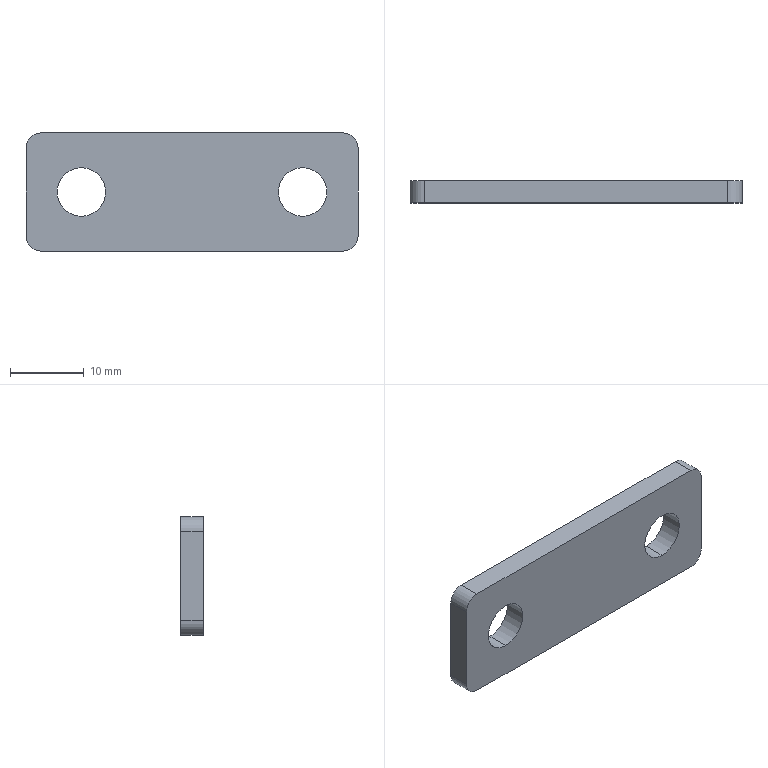Part | STEP file | LM-05-1153A_default | 1 solid | 14 faces | box 45 x 3 x 16 mm | volume 1944 mm3 | cylinder 8 | plane 6 | commonest cylinder face diameters 4 x4 6.6 x4
STEP:
#1=CARTESIAN_POINT('',(0.,0.,0.));
#2=DIRECTION('',(0.,0.,1.));
#3=DIRECTION('',(1.,0.,0.));
#4=AXIS2_PLACEMENT_3D('',#1,#2,#3);
#5=CARTESIAN_POINT('',(15.,-1.5,3.3));
#6=VERTEX_POINT('',#5);
#7=CARTESIAN_POINT('',(15.,1.5,3.3));
#8=VERTEX_POINT('',#7);
#9=CARTESIAN_POINT('',(15.,-1.5,3.3));
#10=DIRECTION('',(0.,1.,0.));
#11=VECTOR('',#10,1.);
#12=LINE('',#9,#11);
#13=CARTESIAN_POINT('',(15.,-1.5,0.));
#14=DIRECTION('',(0.,1.,0.));
#15=DIRECTION('',(0.,0.,1.));
#16=AXIS2_PLACEMENT_3D('',#13,#14,#15);
#17=CYLINDRICAL_SURFACE('',#16,3.3);
#18=CARTESIAN_POINT('',(6.283,0.));
#19=DIRECTION('',(0.,1.));
#20=VECTOR('',#19,1.);
#21=LINE('',#18,#20);
#22=(GEOMETRIC_REPRESENTATION_CONTEXT(2)PARAMETRIC_REPRESENTATION_CONTEXT()REPRESENTATION_CONTEXT('',''));
#23=DEFINITIONAL_REPRESENTATION('',(#21),#22);
#24=PCURVE('',#17,#23);
#25=CARTESIAN_POINT('',(15.,-1.5,0.));
#26=DIRECTION('',(0.,1.,0.));
#27=DIRECTION('',(0.,0.,1.));
#28=AXIS2_PLACEMENT_3D('',#25,#26,#27);
#29=CYLINDRICAL_SURFACE('',#28,3.3);
#30=CARTESIAN_POINT('',(0.,0.));
#31=DIRECTION('',(0.,1.));
#32=VECTOR('',#31,1.);
#33=LINE('',#30,#32);
#34=(GEOMETRIC_REPRESENTATION_CONTEXT(2)PARAMETRIC_REPRESENTATION_CONTEXT()REPRESENTATION_CONTEXT('',''));
#35=DEFINITIONAL_REPRESENTATION('',(#33),#34);
#36=PCURVE('',#29,#35);
#37=SURFACE_CURVE('',#12,(#24,#36),.PCURVE_S1.);
#38=EDGE_CURVE('',#6,#8,#37,.T.);
#39=ORIENTED_EDGE('',*,*,#38,.T.);
#40=CARTESIAN_POINT('',(15.,1.5,-3.3));
#41=VERTEX_POINT('',#40);
#42=CARTESIAN_POINT('',(15.,1.5,0.));
#43=DIRECTION('',(0.,1.,0.));
#44=DIRECTION('',(0.,0.,-1.));
#45=AXIS2_PLACEMENT_3D('',#42,#43,#44);
#46=CIRCLE('',#45,3.3);
#47=CARTESIAN_POINT('',(3.142,3.));
#48=DIRECTION('',(1.,0.));
#49=VECTOR('',#48,1.);
#50=LINE('',#47,#49);
#51=(GEOMETRIC_REPRESENTATION_CONTEXT(2)PARAMETRIC_REPRESENTATION_CONTEXT()REPRESENTATION_CONTEXT('',''));
#52=DEFINITIONAL_REPRESENTATION('',(#50),#51);
#53=PCURVE('',#17,#52);
#54=CARTESIAN_POINT('',(20.5,1.5,-6.));
#55=DIRECTION('',(0.,1.,0.));
#56=DIRECTION('',(0.,0.,1.));
#57=AXIS2_PLACEMENT_3D('',#54,#55,#56);
#58=PLANE('',#57);
#59=CARTESIAN_POINT('',(6.,-5.5));
#60=DIRECTION('',(-1.,0.));
#61=AXIS2_PLACEMENT_2D('',#59,#60);
#62=CIRCLE('',#61,3.3);
#63=(GEOMETRIC_REPRESENTATION_CONTEXT(2)PARAMETRIC_REPRESENTATION_CONTEXT()REPRESENTATION_CONTEXT('',''));
#64=DEFINITIONAL_REPRESENTATION('',(#62),#63);
#65=PCURVE('',#58,#64);
#66=SURFACE_CURVE('',#46,(#53,#65),.PCURVE_S1.);
#67=EDGE_CURVE('',#41,#8,#66,.T.);
#68=ORIENTED_EDGE('',*,*,#67,.F.);
#69=CARTESIAN_POINT('',(15.,-1.5,-3.3));
#70=VERTEX_POINT('',#69);
#71=CARTESIAN_POINT('',(15.,-1.5,-3.3));
#72=DIRECTION('',(0.,1.,0.));
#73=VECTOR('',#72,1.);
#74=LINE('',#71,#73);
#75=CARTESIAN_POINT('',(3.142,0.));
#76=DIRECTION('',(0.,1.));
#77=VECTOR('',#76,1.);
#78=LINE('',#75,#77);
#79=(GEOMETRIC_REPRESENTATION_CONTEXT(2)PARAMETRIC_REPRESENTATION_CONTEXT()REPRESENTATION_CONTEXT('',''));
#80=DEFINITIONAL_REPRESENTATION('',(#78),#79);
#81=PCURVE('',#17,#80);
#82=CARTESIAN_POINT('',(3.142,0.));
#83=DIRECTION('',(0.,1.));
#84=VECTOR('',#83,1.);
#85=LINE('',#82,#84);
#86=(GEOMETRIC_REPRESENTATION_CONTEXT(2)PARAMETRIC_REPRESENTATION_CONTEXT()REPRESENTATION_CONTEXT('',''));
#87=DEFINITIONAL_REPRESENTATION('',(#85),#86);
#88=PCURVE('',#29,#87);
#89=SURFACE_CURVE('',#74,(#81,#88),.PCURVE_S1.);
#90=EDGE_CURVE('',#70,#41,#89,.T.);
#91=ORIENTED_EDGE('',*,*,#90,.F.);
#92=CARTESIAN_POINT('',(15.,-1.5,0.));
#93=DIRECTION('',(0.,1.,0.));
#94=DIRECTION('',(0.,0.,-1.));
#95=AXIS2_PLACEMENT_3D('',#92,#93,#94);
#96=CIRCLE('',#95,3.3);
#97=CARTESIAN_POINT('',(3.142,0.));
#98=DIRECTION('',(1.,0.));
#99=VECTOR('',#98,1.);
#100=LINE('',#97,#99);
#101=(GEOMETRIC_REPRESENTATION_CONTEXT(2)PARAMETRIC_REPRESENTATION_CONTEXT()REPRESENTATION_CONTEXT('',''));
#102=DEFINITIONAL_REPRESENTATION('',(#100),#101);
#103=PCURVE('',#17,#102);
#104=CARTESIAN_POINT('',(20.5,-1.5,-6.));
#105=DIRECTION('',(0.,1.,0.));
#106=DIRECTION('',(0.,0.,1.));
#107=AXIS2_PLACEMENT_3D('',#104,#105,#106);
#108=PLANE('',#107);
#109=CARTESIAN_POINT('',(6.,-5.5));
#110=DIRECTION('',(-1.,0.));
#111=AXIS2_PLACEMENT_2D('',#109,#110);
#112=CIRCLE('',#111,3.3);
#113=(GEOMETRIC_REPRESENTATION_CONTEXT(2)PARAMETRIC_REPRESENTATION_CONTEXT()REPRESENTATION_CONTEXT('',''));
#114=DEFINITIONAL_REPRESENTATION('',(#112),#113);
#115=PCURVE('',#108,#114);
#116=SURFACE_CURVE('',#96,(#103,#115),.PCURVE_S1.);
#117=EDGE_CURVE('',#70,#6,#116,.T.);
#118=ORIENTED_EDGE('',*,*,#117,.T.);
#119=EDGE_LOOP('',(#39,#68,#91,#118));
#120=FACE_BOUND('',#119,.F.);
#121=ADVANCED_FACE('',(#120),#17,.F.);
#122=CARTESIAN_POINT('',(-15.,-1.5,3.3));
#123=VERTEX_POINT('',#122);
#124=CARTESIAN_POINT('',(-15.,1.5,3.3));
#125=VERTEX_POINT('',#124);
#126=CARTESIAN_POINT('',(-15.,-1.5,3.3));
#127=DIRECTION('',(0.,1.,0.));
#128=VECTOR('',#127,1.);
#129=LINE('',#126,#128);
#130=CARTESIAN_POINT('',(-15.,-1.5,0.));
#131=DIRECTION('',(0.,1.,0.));
#132=DIRECTION('',(0.,0.,1.));
#133=AXIS2_PLACEMENT_3D('',#130,#131,#132);
#134=CYLINDRICAL_SURFACE('',#133,3.3);
#135=CARTESIAN_POINT('',(6.283,0.));
#136=DIRECTION('',(0.,1.));
#137=VECTOR('',#136,1.);
#138=LINE('',#135,#137);
#139=(GEOMETRIC_REPRESENTATION_CONTEXT(2)PARAMETRIC_REPRESENTATION_CONTEXT()REPRESENTATION_CONTEXT('',''));
#140=DEFINITIONAL_REPRESENTATION('',(#138),#139);
#141=PCURVE('',#134,#140);
#142=CARTESIAN_POINT('',(-15.,-1.5,0.));
#143=DIRECTION('',(0.,1.,0.));
#144=DIRECTION('',(0.,0.,1.));
#145=AXIS2_PLACEMENT_3D('',#142,#143,#144);
#146=CYLINDRICAL_SURFACE('',#145,3.3);
#147=CARTESIAN_POINT('',(0.,0.));
#148=DIRECTION('',(0.,1.));
#149=VECTOR('',#148,1.);
#150=LINE('',#147,#149);
#151=(GEOMETRIC_REPRESENTATION_CONTEXT(2)PARAMETRIC_REPRESENTATION_CONTEXT()REPRESENTATION_CONTEXT('',''));
#152=DEFINITIONAL_REPRESENTATION('',(#150),#151);
#153=PCURVE('',#146,#152);
#154=SURFACE_CURVE('',#129,(#141,#153),.PCURVE_S1.);
#155=EDGE_CURVE('',#123,#125,#154,.T.);
#156=ORIENTED_EDGE('',*,*,#155,.T.);
#157=CARTESIAN_POINT('',(-15.,1.5,-3.3));
#158=VERTEX_POINT('',#157);
#159=CARTESIAN_POINT('',(-15.,1.5,0.));
#160=DIRECTION('',(0.,1.,0.));
#161=DIRECTION('',(0.,0.,-1.));
#162=AXIS2_PLACEMENT_3D('',#159,#160,#161);
#163=CIRCLE('',#162,3.3);
#164=CARTESIAN_POINT('',(3.142,3.));
#165=DIRECTION('',(1.,0.));
#166=VECTOR('',#165,1.);
#167=LINE('',#164,#166);
#168=(GEOMETRIC_REPRESENTATION_CONTEXT(2)PARAMETRIC_REPRESENTATION_CONTEXT()REPRESENTATION_CONTEXT('',''));
#169=DEFINITIONAL_REPRESENTATION('',(#167),#168);
#170=PCURVE('',#134,#169);
#171=CARTESIAN_POINT('',(6.,-35.5));
#172=DIRECTION('',(-1.,0.));
#173=AXIS2_PLACEMENT_2D('',#171,#172);
#174=CIRCLE('',#173,3.3);
#175=(GEOMETRIC_REPRESENTATION_CONTEXT(2)PARAMETRIC_REPRESENTATION_CONTEXT()REPRESENTATION_CONTEXT('',''));
#176=DEFINITIONAL_REPRESENTATION('',(#174),#175);
#177=PCURVE('',#58,#176);
#178=SURFACE_CURVE('',#163,(#170,#177),.PCURVE_S1.);
#179=EDGE_CURVE('',#158,#125,#178,.T.);
#180=ORIENTED_EDGE('',*,*,#179,.F.);
#181=CARTESIAN_POINT('',(-15.,-1.5,-3.3));
#182=VERTEX_POINT('',#181);
#183=CARTESIAN_POINT('',(-15.,-1.5,-3.3));
#184=DIRECTION('',(0.,1.,0.));
#185=VECTOR('',#184,1.);
#186=LINE('',#183,#185);
#187=CARTESIAN_POINT('',(3.142,0.));
#188=DIRECTION('',(0.,1.));
#189=VECTOR('',#188,1.);
#190=LINE('',#187,#189);
#191=(GEOMETRIC_REPRESENTATION_CONTEXT(2)PARAMETRIC_REPRESENTATION_CONTEXT()REPRESENTATION_CONTEXT('',''));
#192=DEFINITIONAL_REPRESENTATION('',(#190),#191);
#193=PCURVE('',#134,#192);
#194=CARTESIAN_POINT('',(3.142,0.));
#195=DIRECTION('',(0.,1.));
#196=VECTOR('',#195,1.);
#197=LINE('',#194,#196);
#198=(GEOMETRIC_REPRESENTATION_CONTEXT(2)PARAMETRIC_REPRESENTATION_CONTEXT()REPRESENTATION_CONTEXT('',''));
#199=DEFINITIONAL_REPRESENTATION('',(#197),#198);
#200=PCURVE('',#146,#199);
#201=SURFACE_CURVE('',#186,(#193,#200),.PCURVE_S1.);
#202=EDGE_CURVE('',#182,#158,#201,.T.);
#203=ORIENTED_EDGE('',*,*,#202,.F.);
#204=CARTESIAN_POINT('',(-15.,-1.5,0.));
#205=DIRECTION('',(0.,1.,0.));
#206=DIRECTION('',(0.,0.,-1.));
#207=AXIS2_PLACEMENT_3D('',#204,#205,#206);
#208=CIRCLE('',#207,3.3);
#209=CARTESIAN_POINT('',(3.142,0.));
#210=DIRECTION('',(1.,0.));
#211=VECTOR('',#210,1.);
#212=LINE('',#209,#211);
#213=(GEOMETRIC_REPRESENTATION_CONTEXT(2)PARAMETRIC_REPRESENTATION_CONTEXT()REPRESENTATION_CONTEXT('',''));
#214=DEFINITIONAL_REPRESENTATION('',(#212),#213);
#215=PCURVE('',#134,#214);
#216=CARTESIAN_POINT('',(6.,-35.5));
#217=DIRECTION('',(-1.,0.));
#218=AXIS2_PLACEMENT_2D('',#216,#217);
#219=CIRCLE('',#218,3.3);
#220=(GEOMETRIC_REPRESENTATION_CONTEXT(2)PARAMETRIC_REPRESENTATION_CONTEXT()REPRESENTATION_CONTEXT('',''));
#221=DEFINITIONAL_REPRESENTATION('',(#219),#220);
#222=PCURVE('',#108,#221);
#223=SURFACE_CURVE('',#208,(#215,#222),.PCURVE_S1.);
#224=EDGE_CURVE('',#182,#123,#223,.T.);
#225=ORIENTED_EDGE('',*,*,#224,.T.);
#226=EDGE_LOOP('',(#156,#180,#203,#225));
#227=FACE_BOUND('',#226,.F.);
#228=ADVANCED_FACE('',(#227),#134,.F.);
#229=CARTESIAN_POINT('',(22.5,1.5,-6.));
#230=VERTEX_POINT('',#229);
#231=CARTESIAN_POINT('',(20.5,1.5,-8.));
#232=VERTEX_POINT('',#231);
#233=CARTESIAN_POINT('',(20.5,1.5,-6.));
#234=DIRECTION('',(0.,1.,0.));
#235=DIRECTION('',(0.,0.,1.));
#236=AXIS2_PLACEMENT_3D('',#233,#234,#235);
#237=CIRCLE('',#236,2.);
#238=CARTESIAN_POINT('',(20.5,-1.5,-6.));
#239=DIRECTION('',(0.,1.,0.));
#240=DIRECTION('',(0.,0.,1.));
#241=AXIS2_PLACEMENT_3D('',#238,#239,#240);
#242=CYLINDRICAL_SURFACE('',#241,2.);
#243=CARTESIAN_POINT('',(0.,3.));
#244=DIRECTION('',(1.,0.));
#245=VECTOR('',#244,1.);
#246=LINE('',#243,#245);
#247=(GEOMETRIC_REPRESENTATION_CONTEXT(2)PARAMETRIC_REPRESENTATION_CONTEXT()REPRESENTATION_CONTEXT('',''));
#248=DEFINITIONAL_REPRESENTATION('',(#246),#247);
#249=PCURVE('',#242,#248);
#250=CARTESIAN_POINT('',(0.,0.));
#251=DIRECTION('',(1.,0.));
#252=AXIS2_PLACEMENT_2D('',#250,#251);
#253=CIRCLE('',#252,2.);
#254=(GEOMETRIC_REPRESENTATION_CONTEXT(2)PARAMETRIC_REPRESENTATION_CONTEXT()REPRESENTATION_CONTEXT('',''));
#255=DEFINITIONAL_REPRESENTATION('',(#253),#254);
#256=PCURVE('',#58,#255);
#257=SURFACE_CURVE('',#237,(#249,#256),.PCURVE_S1.);
#258=EDGE_CURVE('',#230,#232,#257,.T.);
#259=ORIENTED_EDGE('',*,*,#258,.F.);
#260=CARTESIAN_POINT('',(22.5,-1.5,-6.));
#261=VERTEX_POINT('',#260);
#262=CARTESIAN_POINT('',(22.5,-1.5,-6.));
#263=DIRECTION('',(0.,1.,0.));
#264=VECTOR('',#263,1.);
#265=LINE('',#262,#264);
#266=CARTESIAN_POINT('',(1.571,0.));
#267=DIRECTION('',(0.,1.));
#268=VECTOR('',#267,1.);
#269=LINE('',#266,#268);
#270=(GEOMETRIC_REPRESENTATION_CONTEXT(2)PARAMETRIC_REPRESENTATION_CONTEXT()REPRESENTATION_CONTEXT('',''));
#271=DEFINITIONAL_REPRESENTATION('',(#269),#270);
#272=PCURVE('',#242,#271);
#273=CARTESIAN_POINT('',(22.5,-1.5,6.));
#274=DIRECTION('',(1.,0.,0.));
#275=DIRECTION('',(0.,0.,-1.));
#276=AXIS2_PLACEMENT_3D('',#273,#274,#275);
#277=PLANE('',#276);
#278=CARTESIAN_POINT('',(12.,0.));
#279=DIRECTION('',(0.,1.));
#280=VECTOR('',#279,1.);
#281=LINE('',#278,#280);
#282=(GEOMETRIC_REPRESENTATION_CONTEXT(2)PARAMETRIC_REPRESENTATION_CONTEXT()REPRESENTATION_CONTEXT('',''));
#283=DEFINITIONAL_REPRESENTATION('',(#281),#282);
#284=PCURVE('',#277,#283);
#285=SURFACE_CURVE('',#265,(#272,#284),.PCURVE_S1.);
#286=EDGE_CURVE('',#261,#230,#285,.T.);
#287=ORIENTED_EDGE('',*,*,#286,.F.);
#288=CARTESIAN_POINT('',(20.5,-1.5,-8.));
#289=VERTEX_POINT('',#288);
#290=CARTESIAN_POINT('',(20.5,-1.5,-6.));
#291=DIRECTION('',(0.,1.,0.));
#292=DIRECTION('',(0.,0.,1.));
#293=AXIS2_PLACEMENT_3D('',#290,#291,#292);
#294=CIRCLE('',#293,2.);
#295=CARTESIAN_POINT('',(0.,0.));
#296=DIRECTION('',(1.,0.));
#297=VECTOR('',#296,1.);
#298=LINE('',#295,#297);
#299=(GEOMETRIC_REPRESENTATION_CONTEXT(2)PARAMETRIC_REPRESENTATION_CONTEXT()REPRESENTATION_CONTEXT('',''));
#300=DEFINITIONAL_REPRESENTATION('',(#298),#299);
#301=PCURVE('',#242,#300);
#302=CARTESIAN_POINT('',(0.,0.));
#303=DIRECTION('',(1.,0.));
#304=AXIS2_PLACEMENT_2D('',#302,#303);
#305=CIRCLE('',#304,2.);
#306=(GEOMETRIC_REPRESENTATION_CONTEXT(2)PARAMETRIC_REPRESENTATION_CONTEXT()REPRESENTATION_CONTEXT('',''));
#307=DEFINITIONAL_REPRESENTATION('',(#305),#306);
#308=PCURVE('',#108,#307);
#309=SURFACE_CURVE('',#294,(#301,#308),.PCURVE_S1.);
#310=EDGE_CURVE('',#261,#289,#309,.T.);
#311=ORIENTED_EDGE('',*,*,#310,.T.);
#312=CARTESIAN_POINT('',(20.5,-1.5,-8.));
#313=DIRECTION('',(0.,1.,0.));
#314=VECTOR('',#313,1.);
#315=LINE('',#312,#314);
#316=CARTESIAN_POINT('',(3.142,0.));
#317=DIRECTION('',(0.,1.));
#318=VECTOR('',#317,1.);
#319=LINE('',#316,#318);
#320=(GEOMETRIC_REPRESENTATION_CONTEXT(2)PARAMETRIC_REPRESENTATION_CONTEXT()REPRESENTATION_CONTEXT('',''));
#321=DEFINITIONAL_REPRESENTATION('',(#319),#320);
#322=PCURVE('',#242,#321);
#323=CARTESIAN_POINT('',(20.5,-1.5,-8.));
#324=DIRECTION('',(0.,0.,-1.));
#325=DIRECTION('',(-1.,0.,0.));
#326=AXIS2_PLACEMENT_3D('',#323,#324,#325);
#327=PLANE('',#326);
#328=CARTESIAN_POINT('',(0.,0.));
#329=DIRECTION('',(0.,1.));
#330=VECTOR('',#329,1.);
#331=LINE('',#328,#330);
#332=(GEOMETRIC_REPRESENTATION_CONTEXT(2)PARAMETRIC_REPRESENTATION_CONTEXT()REPRESENTATION_CONTEXT('',''));
#333=DEFINITIONAL_REPRESENTATION('',(#331),#332);
#334=PCURVE('',#327,#333);
#335=SURFACE_CURVE('',#315,(#322,#334),.PCURVE_S1.);
#336=EDGE_CURVE('',#289,#232,#335,.T.);
#337=ORIENTED_EDGE('',*,*,#336,.T.);
#338=EDGE_LOOP('',(#259,#287,#311,#337));
#339=FACE_BOUND('',#338,.T.);
#340=ADVANCED_FACE('',(#339),#242,.T.);
#341=CARTESIAN_POINT('',(22.5,1.5,6.));
#342=VERTEX_POINT('',#341);
#343=CARTESIAN_POINT('',(22.5,1.5,6.));
#344=DIRECTION('',(0.,0.,-1.));
#345=VECTOR('',#344,1.);
#346=LINE('',#343,#345);
#347=CARTESIAN_POINT('',(0.,3.));
#348=DIRECTION('',(1.,0.));
#349=VECTOR('',#348,1.);
#350=LINE('',#347,#349);
#351=(GEOMETRIC_REPRESENTATION_CONTEXT(2)PARAMETRIC_REPRESENTATION_CONTEXT()REPRESENTATION_CONTEXT('',''));
#352=DEFINITIONAL_REPRESENTATION('',(#350),#351);
#353=PCURVE('',#277,#352);
#354=CARTESIAN_POINT('',(12.,2.));
#355=DIRECTION('',(-1.,0.));
#356=VECTOR('',#355,1.);
#357=LINE('',#354,#356);
#358=(GEOMETRIC_REPRESENTATION_CONTEXT(2)PARAMETRIC_REPRESENTATION_CONTEXT()REPRESENTATION_CONTEXT('',''));
#359=DEFINITIONAL_REPRESENTATION('',(#357),#358);
#360=PCURVE('',#58,#359);
#361=SURFACE_CURVE('',#346,(#353,#360),.PCURVE_S1.);
#362=EDGE_CURVE('',#342,#230,#361,.T.);
#363=ORIENTED_EDGE('',*,*,#362,.F.);
#364=CARTESIAN_POINT('',(22.5,-1.5,6.));
#365=VERTEX_POINT('',#364);
#366=CARTESIAN_POINT('',(22.5,-1.5,6.));
#367=DIRECTION('',(0.,1.,0.));
#368=VECTOR('',#367,1.);
#369=LINE('',#366,#368);
#370=CARTESIAN_POINT('',(0.,0.));
#371=DIRECTION('',(0.,1.));
#372=VECTOR('',#371,1.);
#373=LINE('',#370,#372);
#374=(GEOMETRIC_REPRESENTATION_CONTEXT(2)PARAMETRIC_REPRESENTATION_CONTEXT()REPRESENTATION_CONTEXT('',''));
#375=DEFINITIONAL_REPRESENTATION('',(#373),#374);
#376=PCURVE('',#277,#375);
#377=CARTESIAN_POINT('',(20.5,-1.5,6.));
#378=DIRECTION('',(0.,1.,0.));
#379=DIRECTION('',(0.,0.,1.));
#380=AXIS2_PLACEMENT_3D('',#377,#378,#379);
#381=CYLINDRICAL_SURFACE('',#380,2.);
#382=CARTESIAN_POINT('',(1.571,0.));
#383=DIRECTION('',(0.,1.));
#384=VECTOR('',#383,1.);
#385=LINE('',#382,#384);
#386=(GEOMETRIC_REPRESENTATION_CONTEXT(2)PARAMETRIC_REPRESENTATION_CONTEXT()REPRESENTATION_CONTEXT('',''));
#387=DEFINITIONAL_REPRESENTATION('',(#385),#386);
#388=PCURVE('',#381,#387);
#389=SURFACE_CURVE('',#369,(#376,#388),.PCURVE_S1.);
#390=EDGE_CURVE('',#365,#342,#389,.T.);
#391=ORIENTED_EDGE('',*,*,#390,.F.);
#392=CARTESIAN_POINT('',(22.5,-1.5,6.));
#393=DIRECTION('',(0.,0.,-1.));
#394=VECTOR('',#393,1.);
#395=LINE('',#392,#394);
#396=CARTESIAN_POINT('',(0.,0.));
#397=DIRECTION('',(1.,0.));
#398=VECTOR('',#397,1.);
#399=LINE('',#396,#398);
#400=(GEOMETRIC_REPRESENTATION_CONTEXT(2)PARAMETRIC_REPRESENTATION_CONTEXT()REPRESENTATION_CONTEXT('',''));
#401=DEFINITIONAL_REPRESENTATION('',(#399),#400);
#402=PCURVE('',#277,#401);
#403=CARTESIAN_POINT('',(12.,2.));
#404=DIRECTION('',(-1.,0.));
#405=VECTOR('',#404,1.);
#406=LINE('',#403,#405);
#407=(GEOMETRIC_REPRESENTATION_CONTEXT(2)PARAMETRIC_REPRESENTATION_CONTEXT()REPRESENTATION_CONTEXT('',''));
#408=DEFINITIONAL_REPRESENTATION('',(#406),#407);
#409=PCURVE('',#108,#408);
#410=SURFACE_CURVE('',#395,(#402,#409),.PCURVE_S1.);
#411=EDGE_CURVE('',#365,#261,#410,.T.);
#412=ORIENTED_EDGE('',*,*,#411,.T.);
#413=ORIENTED_EDGE('',*,*,#286,.T.);
#414=EDGE_LOOP('',(#363,#391,#412,#413));
#415=FACE_BOUND('',#414,.T.);
#416=ADVANCED_FACE('',(#415),#277,.T.);
#417=CARTESIAN_POINT('',(20.5,1.5,8.));
#418=VERTEX_POINT('',#417);
#419=CARTESIAN_POINT('',(20.5,1.5,6.));
#420=DIRECTION('',(0.,1.,0.));
#421=DIRECTION('',(0.,0.,1.));
#422=AXIS2_PLACEMENT_3D('',#419,#420,#421);
#423=CIRCLE('',#422,2.);
#424=CARTESIAN_POINT('',(0.,3.));
#425=DIRECTION('',(1.,0.));
#426=VECTOR('',#425,1.);
#427=LINE('',#424,#426);
#428=(GEOMETRIC_REPRESENTATION_CONTEXT(2)PARAMETRIC_REPRESENTATION_CONTEXT()REPRESENTATION_CONTEXT('',''));
#429=DEFINITIONAL_REPRESENTATION('',(#427),#428);
#430=PCURVE('',#381,#429);
#431=CARTESIAN_POINT('',(12.,0.));
#432=DIRECTION('',(1.,0.));
#433=AXIS2_PLACEMENT_2D('',#431,#432);
#434=CIRCLE('',#433,2.);
#435=(GEOMETRIC_REPRESENTATION_CONTEXT(2)PARAMETRIC_REPRESENTATION_CONTEXT()REPRESENTATION_CONTEXT('',''));
#436=DEFINITIONAL_REPRESENTATION('',(#434),#435);
#437=PCURVE('',#58,#436);
#438=SURFACE_CURVE('',#423,(#430,#437),.PCURVE_S1.);
#439=EDGE_CURVE('',#418,#342,#438,.T.);
#440=ORIENTED_EDGE('',*,*,#439,.F.);
#441=CARTESIAN_POINT('',(20.5,-1.5,8.));
#442=VERTEX_POINT('',#441);
#443=CARTESIAN_POINT('',(20.5,-1.5,8.));
#444=DIRECTION('',(0.,1.,0.));
#445=VECTOR('',#444,1.);
#446=LINE('',#443,#445);
#447=CARTESIAN_POINT('',(0.,0.));
#448=DIRECTION('',(0.,1.));
#449=VECTOR('',#448,1.);
#450=LINE('',#447,#449);
#451=(GEOMETRIC_REPRESENTATION_CONTEXT(2)PARAMETRIC_REPRESENTATION_CONTEXT()REPRESENTATION_CONTEXT('',''));
#452=DEFINITIONAL_REPRESENTATION('',(#450),#451);
#453=PCURVE('',#381,#452);
#454=CARTESIAN_POINT('',(-20.5,-1.5,8.));
#455=DIRECTION('',(0.,0.,1.));
#456=DIRECTION('',(1.,0.,0.));
#457=AXIS2_PLACEMENT_3D('',#454,#455,#456);
#458=PLANE('',#457);
#459=CARTESIAN_POINT('',(41.,0.));
#460=DIRECTION('',(0.,1.));
#461=VECTOR('',#460,1.);
#462=LINE('',#459,#461);
#463=(GEOMETRIC_REPRESENTATION_CONTEXT(2)PARAMETRIC_REPRESENTATION_CONTEXT()REPRESENTATION_CONTEXT('',''));
#464=DEFINITIONAL_REPRESENTATION('',(#462),#463);
#465=PCURVE('',#458,#464);
#466=SURFACE_CURVE('',#446,(#453,#465),.PCURVE_S1.);
#467=EDGE_CURVE('',#442,#418,#466,.T.);
#468=ORIENTED_EDGE('',*,*,#467,.F.);
#469=CARTESIAN_POINT('',(20.5,-1.5,6.));
#470=DIRECTION('',(0.,1.,0.));
#471=DIRECTION('',(0.,0.,1.));
#472=AXIS2_PLACEMENT_3D('',#469,#470,#471);
#473=CIRCLE('',#472,2.);
#474=CARTESIAN_POINT('',(0.,0.));
#475=DIRECTION('',(1.,0.));
#476=VECTOR('',#475,1.);
#477=LINE('',#474,#476);
#478=(GEOMETRIC_REPRESENTATION_CONTEXT(2)PARAMETRIC_REPRESENTATION_CONTEXT()REPRESENTATION_CONTEXT('',''));
#479=DEFINITIONAL_REPRESENTATION('',(#477),#478);
#480=PCURVE('',#381,#479);
#481=CARTESIAN_POINT('',(12.,0.));
#482=DIRECTION('',(1.,0.));
#483=AXIS2_PLACEMENT_2D('',#481,#482);
#484=CIRCLE('',#483,2.);
#485=(GEOMETRIC_REPRESENTATION_CONTEXT(2)PARAMETRIC_REPRESENTATION_CONTEXT()REPRESENTATION_CONTEXT('',''));
#486=DEFINITIONAL_REPRESENTATION('',(#484),#485);
#487=PCURVE('',#108,#486);
#488=SURFACE_CURVE('',#473,(#480,#487),.PCURVE_S1.);
#489=EDGE_CURVE('',#442,#365,#488,.T.);
#490=ORIENTED_EDGE('',*,*,#489,.T.);
#491=ORIENTED_EDGE('',*,*,#390,.T.);
#492=EDGE_LOOP('',(#440,#468,#490,#491));
#493=FACE_BOUND('',#492,.T.);
#494=ADVANCED_FACE('',(#493),#381,.T.);
#495=CARTESIAN_POINT('',(-20.5,1.5,8.));
#496=VERTEX_POINT('',#495);
#497=CARTESIAN_POINT('',(-20.5,1.5,8.));
#498=DIRECTION('',(1.,0.,0.));
#499=VECTOR('',#498,1.);
#500=LINE('',#497,#499);
#501=CARTESIAN_POINT('',(0.,3.));
#502=DIRECTION('',(1.,0.));
#503=VECTOR('',#502,1.);
#504=LINE('',#501,#503);
#505=(GEOMETRIC_REPRESENTATION_CONTEXT(2)PARAMETRIC_REPRESENTATION_CONTEXT()REPRESENTATION_CONTEXT('',''));
#506=DEFINITIONAL_REPRESENTATION('',(#504),#505);
#507=PCURVE('',#458,#506);
#508=CARTESIAN_POINT('',(14.,-41.));
#509=DIRECTION('',(0.,1.));
#510=VECTOR('',#509,1.);
#511=LINE('',#508,#510);
#512=(GEOMETRIC_REPRESENTATION_CONTEXT(2)PARAMETRIC_REPRESENTATION_CONTEXT()REPRESENTATION_CONTEXT('',''));
#513=DEFINITIONAL_REPRESENTATION('',(#511),#512);
#514=PCURVE('',#58,#513);
#515=SURFACE_CURVE('',#500,(#507,#514),.PCURVE_S1.);
#516=EDGE_CURVE('',#496,#418,#515,.T.);
#517=ORIENTED_EDGE('',*,*,#516,.F.);
#518=CARTESIAN_POINT('',(-20.5,-1.5,8.));
#519=VERTEX_POINT('',#518);
#520=CARTESIAN_POINT('',(-20.5,-1.5,8.));
#521=DIRECTION('',(0.,1.,0.));
#522=VECTOR('',#521,1.);
#523=LINE('',#520,#522);
#524=CARTESIAN_POINT('',(0.,0.));
#525=DIRECTION('',(0.,1.));
#526=VECTOR('',#525,1.);
#527=LINE('',#524,#526);
#528=(GEOMETRIC_REPRESENTATION_CONTEXT(2)PARAMETRIC_REPRESENTATION_CONTEXT()REPRESENTATION_CONTEXT('',''));
#529=DEFINITIONAL_REPRESENTATION('',(#527),#528);
#530=PCURVE('',#458,#529);
#531=CARTESIAN_POINT('',(-20.5,-1.5,6.));
#532=DIRECTION('',(0.,1.,0.));
#533=DIRECTION('',(0.,0.,1.));
#534=AXIS2_PLACEMENT_3D('',#531,#532,#533);
#535=CYLINDRICAL_SURFACE('',#534,2.);
#536=CARTESIAN_POINT('',(6.283,0.));
#537=DIRECTION('',(0.,1.));
#538=VECTOR('',#537,1.);
#539=LINE('',#536,#538);
#540=(GEOMETRIC_REPRESENTATION_CONTEXT(2)PARAMETRIC_REPRESENTATION_CONTEXT()REPRESENTATION_CONTEXT('',''));
#541=DEFINITIONAL_REPRESENTATION('',(#539),#540);
#542=PCURVE('',#535,#541);
#543=SURFACE_CURVE('',#523,(#530,#542),.PCURVE_S1.);
#544=EDGE_CURVE('',#519,#496,#543,.T.);
#545=ORIENTED_EDGE('',*,*,#544,.F.);
#546=CARTESIAN_POINT('',(-20.5,-1.5,8.));
#547=DIRECTION('',(1.,0.,0.));
#548=VECTOR('',#547,1.);
#549=LINE('',#546,#548);
#550=CARTESIAN_POINT('',(0.,0.));
#551=DIRECTION('',(1.,0.));
#552=VECTOR('',#551,1.);
#553=LINE('',#550,#552);
#554=(GEOMETRIC_REPRESENTATION_CONTEXT(2)PARAMETRIC_REPRESENTATION_CONTEXT()REPRESENTATION_CONTEXT('',''));
#555=DEFINITIONAL_REPRESENTATION('',(#553),#554);
#556=PCURVE('',#458,#555);
#557=CARTESIAN_POINT('',(14.,-41.));
#558=DIRECTION('',(0.,1.));
#559=VECTOR('',#558,1.);
#560=LINE('',#557,#559);
#561=(GEOMETRIC_REPRESENTATION_CONTEXT(2)PARAMETRIC_REPRESENTATION_CONTEXT()REPRESENTATION_CONTEXT('',''));
#562=DEFINITIONAL_REPRESENTATION('',(#560),#561);
#563=PCURVE('',#108,#562);
#564=SURFACE_CURVE('',#549,(#556,#563),.PCURVE_S1.);
#565=EDGE_CURVE('',#519,#442,#564,.T.);
#566=ORIENTED_EDGE('',*,*,#565,.T.);
#567=ORIENTED_EDGE('',*,*,#467,.T.);
#568=EDGE_LOOP('',(#517,#545,#566,#567));
#569=FACE_BOUND('',#568,.T.);
#570=ADVANCED_FACE('',(#569),#458,.T.);
#571=CARTESIAN_POINT('',(-22.5,1.5,6.));
#572=VERTEX_POINT('',#571);
#573=CARTESIAN_POINT('',(-20.5,1.5,6.));
#574=DIRECTION('',(0.,1.,0.));
#575=DIRECTION('',(0.,0.,1.));
#576=AXIS2_PLACEMENT_3D('',#573,#574,#575);
#577=CIRCLE('',#576,2.);
#578=CARTESIAN_POINT('',(0.,3.));
#579=DIRECTION('',(1.,0.));
#580=VECTOR('',#579,1.);
#581=LINE('',#578,#580);
#582=(GEOMETRIC_REPRESENTATION_CONTEXT(2)PARAMETRIC_REPRESENTATION_CONTEXT()REPRESENTATION_CONTEXT('',''));
#583=DEFINITIONAL_REPRESENTATION('',(#581),#582);
#584=PCURVE('',#535,#583);
#585=CARTESIAN_POINT('',(12.,-41.));
#586=DIRECTION('',(1.,0.));
#587=AXIS2_PLACEMENT_2D('',#585,#586);
#588=CIRCLE('',#587,2.);
#589=(GEOMETRIC_REPRESENTATION_CONTEXT(2)PARAMETRIC_REPRESENTATION_CONTEXT()REPRESENTATION_CONTEXT('',''));
#590=DEFINITIONAL_REPRESENTATION('',(#588),#589);
#591=PCURVE('',#58,#590);
#592=SURFACE_CURVE('',#577,(#584,#591),.PCURVE_S1.);
#593=EDGE_CURVE('',#572,#496,#592,.T.);
#594=ORIENTED_EDGE('',*,*,#593,.F.);
#595=CARTESIAN_POINT('',(-22.5,-1.5,6.));
#596=VERTEX_POINT('',#595);
#597=CARTESIAN_POINT('',(-22.5,-1.5,6.));
#598=DIRECTION('',(0.,1.,0.));
#599=VECTOR('',#598,1.);
#600=LINE('',#597,#599);
#601=CARTESIAN_POINT('',(4.712,0.));
#602=DIRECTION('',(0.,1.));
#603=VECTOR('',#602,1.);
#604=LINE('',#601,#603);
#605=(GEOMETRIC_REPRESENTATION_CONTEXT(2)PARAMETRIC_REPRESENTATION_CONTEXT()REPRESENTATION_CONTEXT('',''));
#606=DEFINITIONAL_REPRESENTATION('',(#604),#605);
#607=PCURVE('',#535,#606);
#608=CARTESIAN_POINT('',(-22.5,-1.5,-6.));
#609=DIRECTION('',(-1.,0.,0.));
#610=DIRECTION('',(0.,0.,1.));
#611=AXIS2_PLACEMENT_3D('',#608,#609,#610);
#612=PLANE('',#611);
#613=CARTESIAN_POINT('',(12.,0.));
#614=DIRECTION('',(0.,1.));
#615=VECTOR('',#614,1.);
#616=LINE('',#613,#615);
#617=(GEOMETRIC_REPRESENTATION_CONTEXT(2)PARAMETRIC_REPRESENTATION_CONTEXT()REPRESENTATION_CONTEXT('',''));
#618=DEFINITIONAL_REPRESENTATION('',(#616),#617);
#619=PCURVE('',#612,#618);
#620=SURFACE_CURVE('',#600,(#607,#619),.PCURVE_S1.);
#621=EDGE_CURVE('',#596,#572,#620,.T.);
#622=ORIENTED_EDGE('',*,*,#621,.F.);
#623=CARTESIAN_POINT('',(-20.5,-1.5,6.));
#624=DIRECTION('',(0.,1.,0.));
#625=DIRECTION('',(0.,0.,1.));
#626=AXIS2_PLACEMENT_3D('',#623,#624,#625);
#627=CIRCLE('',#626,2.);
#628=CARTESIAN_POINT('',(0.,0.));
#629=DIRECTION('',(1.,0.));
#630=VECTOR('',#629,1.);
#631=LINE('',#628,#630);
#632=(GEOMETRIC_REPRESENTATION_CONTEXT(2)PARAMETRIC_REPRESENTATION_CONTEXT()REPRESENTATION_CONTEXT('',''));
#633=DEFINITIONAL_REPRESENTATION('',(#631),#632);
#634=PCURVE('',#535,#633);
#635=CARTESIAN_POINT('',(12.,-41.));
#636=DIRECTION('',(1.,0.));
#637=AXIS2_PLACEMENT_2D('',#635,#636);
#638=CIRCLE('',#637,2.);
#639=(GEOMETRIC_REPRESENTATION_CONTEXT(2)PARAMETRIC_REPRESENTATION_CONTEXT()REPRESENTATION_CONTEXT('',''));
#640=DEFINITIONAL_REPRESENTATION('',(#638),#639);
#641=PCURVE('',#108,#640);
#642=SURFACE_CURVE('',#627,(#634,#641),.PCURVE_S1.);
#643=EDGE_CURVE('',#596,#519,#642,.T.);
#644=ORIENTED_EDGE('',*,*,#643,.T.);
#645=ORIENTED_EDGE('',*,*,#544,.T.);
#646=EDGE_LOOP('',(#594,#622,#644,#645));
#647=FACE_BOUND('',#646,.T.);
#648=ADVANCED_FACE('',(#647),#535,.T.);
#649=CARTESIAN_POINT('',(-22.5,1.5,-6.));
#650=VERTEX_POINT('',#649);
#651=CARTESIAN_POINT('',(-22.5,1.5,-6.));
#652=DIRECTION('',(0.,0.,1.));
#653=VECTOR('',#652,1.);
#654=LINE('',#651,#653);
#655=CARTESIAN_POINT('',(0.,3.));
#656=DIRECTION('',(1.,0.));
#657=VECTOR('',#656,1.);
#658=LINE('',#655,#657);
#659=(GEOMETRIC_REPRESENTATION_CONTEXT(2)PARAMETRIC_REPRESENTATION_CONTEXT()REPRESENTATION_CONTEXT('',''));
#660=DEFINITIONAL_REPRESENTATION('',(#658),#659);
#661=PCURVE('',#612,#660);
#662=CARTESIAN_POINT('',(0.,-43.));
#663=DIRECTION('',(1.,0.));
#664=VECTOR('',#663,1.);
#665=LINE('',#662,#664);
#666=(GEOMETRIC_REPRESENTATION_CONTEXT(2)PARAMETRIC_REPRESENTATION_CONTEXT()REPRESENTATION_CONTEXT('',''));
#667=DEFINITIONAL_REPRESENTATION('',(#665),#666);
#668=PCURVE('',#58,#667);
#669=SURFACE_CURVE('',#654,(#661,#668),.PCURVE_S1.);
#670=EDGE_CURVE('',#650,#572,#669,.T.);
#671=ORIENTED_EDGE('',*,*,#670,.F.);
#672=CARTESIAN_POINT('',(-22.5,-1.5,-6.));
#673=VERTEX_POINT('',#672);
#674=CARTESIAN_POINT('',(-22.5,-1.5,-6.));
#675=DIRECTION('',(0.,1.,0.));
#676=VECTOR('',#675,1.);
#677=LINE('',#674,#676);
#678=CARTESIAN_POINT('',(0.,0.));
#679=DIRECTION('',(0.,1.));
#680=VECTOR('',#679,1.);
#681=LINE('',#678,#680);
#682=(GEOMETRIC_REPRESENTATION_CONTEXT(2)PARAMETRIC_REPRESENTATION_CONTEXT()REPRESENTATION_CONTEXT('',''));
#683=DEFINITIONAL_REPRESENTATION('',(#681),#682);
#684=PCURVE('',#612,#683);
#685=CARTESIAN_POINT('',(-20.5,-1.5,-6.));
#686=DIRECTION('',(0.,1.,0.));
#687=DIRECTION('',(0.,0.,1.));
#688=AXIS2_PLACEMENT_3D('',#685,#686,#687);
#689=CYLINDRICAL_SURFACE('',#688,2.);
#690=CARTESIAN_POINT('',(4.712,0.));
#691=DIRECTION('',(0.,1.));
#692=VECTOR('',#691,1.);
#693=LINE('',#690,#692);
#694=(GEOMETRIC_REPRESENTATION_CONTEXT(2)PARAMETRIC_REPRESENTATION_CONTEXT()REPRESENTATION_CONTEXT('',''));
#695=DEFINITIONAL_REPRESENTATION('',(#693),#694);
#696=PCURVE('',#689,#695);
#697=SURFACE_CURVE('',#677,(#684,#696),.PCURVE_S1.);
#698=EDGE_CURVE('',#673,#650,#697,.T.);
#699=ORIENTED_EDGE('',*,*,#698,.F.);
#700=CARTESIAN_POINT('',(-22.5,-1.5,-6.));
#701=DIRECTION('',(0.,0.,1.));
#702=VECTOR('',#701,1.);
#703=LINE('',#700,#702);
#704=CARTESIAN_POINT('',(0.,0.));
#705=DIRECTION('',(1.,0.));
#706=VECTOR('',#705,1.);
#707=LINE('',#704,#706);
#708=(GEOMETRIC_REPRESENTATION_CONTEXT(2)PARAMETRIC_REPRESENTATION_CONTEXT()REPRESENTATION_CONTEXT('',''));
#709=DEFINITIONAL_REPRESENTATION('',(#707),#708);
#710=PCURVE('',#612,#709);
#711=CARTESIAN_POINT('',(0.,-43.));
#712=DIRECTION('',(1.,0.));
#713=VECTOR('',#712,1.);
#714=LINE('',#711,#713);
#715=(GEOMETRIC_REPRESENTATION_CONTEXT(2)PARAMETRIC_REPRESENTATION_CONTEXT()REPRESENTATION_CONTEXT('',''));
#716=DEFINITIONAL_REPRESENTATION('',(#714),#715);
#717=PCURVE('',#108,#716);
#718=SURFACE_CURVE('',#703,(#710,#717),.PCURVE_S1.);
#719=EDGE_CURVE('',#673,#596,#718,.T.);
#720=ORIENTED_EDGE('',*,*,#719,.T.);
#721=ORIENTED_EDGE('',*,*,#621,.T.);
#722=EDGE_LOOP('',(#671,#699,#720,#721));
#723=FACE_BOUND('',#722,.T.);
#724=ADVANCED_FACE('',(#723),#612,.T.);
#725=CARTESIAN_POINT('',(-20.5,1.5,-8.));
#726=VERTEX_POINT('',#725);
#727=CARTESIAN_POINT('',(-20.5,1.5,-6.));
#728=DIRECTION('',(0.,1.,0.));
#729=DIRECTION('',(0.,0.,1.));
#730=AXIS2_PLACEMENT_3D('',#727,#728,#729);
#731=CIRCLE('',#730,2.);
#732=CARTESIAN_POINT('',(0.,3.));
#733=DIRECTION('',(1.,0.));
#734=VECTOR('',#733,1.);
#735=LINE('',#732,#734);
#736=(GEOMETRIC_REPRESENTATION_CONTEXT(2)PARAMETRIC_REPRESENTATION_CONTEXT()REPRESENTATION_CONTEXT('',''));
#737=DEFINITIONAL_REPRESENTATION('',(#735),#736);
#738=PCURVE('',#689,#737);
#739=CARTESIAN_POINT('',(0.,-41.));
#740=DIRECTION('',(1.,0.));
#741=AXIS2_PLACEMENT_2D('',#739,#740);
#742=CIRCLE('',#741,2.);
#743=(GEOMETRIC_REPRESENTATION_CONTEXT(2)PARAMETRIC_REPRESENTATION_CONTEXT()REPRESENTATION_CONTEXT('',''));
#744=DEFINITIONAL_REPRESENTATION('',(#742),#743);
#745=PCURVE('',#58,#744);
#746=SURFACE_CURVE('',#731,(#738,#745),.PCURVE_S1.);
#747=EDGE_CURVE('',#726,#650,#746,.T.);
#748=ORIENTED_EDGE('',*,*,#747,.F.);
#749=CARTESIAN_POINT('',(-20.5,-1.5,-8.));
#750=VERTEX_POINT('',#749);
#751=CARTESIAN_POINT('',(-20.5,-1.5,-8.));
#752=DIRECTION('',(0.,1.,0.));
#753=VECTOR('',#752,1.);
#754=LINE('',#751,#753);
#755=CARTESIAN_POINT('',(3.142,0.));
#756=DIRECTION('',(0.,1.));
#757=VECTOR('',#756,1.);
#758=LINE('',#755,#757);
#759=(GEOMETRIC_REPRESENTATION_CONTEXT(2)PARAMETRIC_REPRESENTATION_CONTEXT()REPRESENTATION_CONTEXT('',''));
#760=DEFINITIONAL_REPRESENTATION('',(#758),#759);
#761=PCURVE('',#689,#760);
#762=CARTESIAN_POINT('',(41.,0.));
#763=DIRECTION('',(0.,1.));
#764=VECTOR('',#763,1.);
#765=LINE('',#762,#764);
#766=(GEOMETRIC_REPRESENTATION_CONTEXT(2)PARAMETRIC_REPRESENTATION_CONTEXT()REPRESENTATION_CONTEXT('',''));
#767=DEFINITIONAL_REPRESENTATION('',(#765),#766);
#768=PCURVE('',#327,#767);
#769=SURFACE_CURVE('',#754,(#761,#768),.PCURVE_S1.);
#770=EDGE_CURVE('',#750,#726,#769,.T.);
#771=ORIENTED_EDGE('',*,*,#770,.F.);
#772=CARTESIAN_POINT('',(-20.5,-1.5,-6.));
#773=DIRECTION('',(0.,1.,0.));
#774=DIRECTION('',(0.,0.,1.));
#775=AXIS2_PLACEMENT_3D('',#772,#773,#774);
#776=CIRCLE('',#775,2.);
#777=CARTESIAN_POINT('',(0.,0.));
#778=DIRECTION('',(1.,0.));
#779=VECTOR('',#778,1.);
#780=LINE('',#777,#779);
#781=(GEOMETRIC_REPRESENTATION_CONTEXT(2)PARAMETRIC_REPRESENTATION_CONTEXT()REPRESENTATION_CONTEXT('',''));
#782=DEFINITIONAL_REPRESENTATION('',(#780),#781);
#783=PCURVE('',#689,#782);
#784=CARTESIAN_POINT('',(0.,-41.));
#785=DIRECTION('',(1.,0.));
#786=AXIS2_PLACEMENT_2D('',#784,#785);
#787=CIRCLE('',#786,2.);
#788=(GEOMETRIC_REPRESENTATION_CONTEXT(2)PARAMETRIC_REPRESENTATION_CONTEXT()REPRESENTATION_CONTEXT('',''));
#789=DEFINITIONAL_REPRESENTATION('',(#787),#788);
#790=PCURVE('',#108,#789);
#791=SURFACE_CURVE('',#776,(#783,#790),.PCURVE_S1.);
#792=EDGE_CURVE('',#750,#673,#791,.T.);
#793=ORIENTED_EDGE('',*,*,#792,.T.);
#794=ORIENTED_EDGE('',*,*,#698,.T.);
#795=EDGE_LOOP('',(#748,#771,#793,#794));
#796=FACE_BOUND('',#795,.T.);
#797=ADVANCED_FACE('',(#796),#689,.T.);
#798=CARTESIAN_POINT('',(20.5,1.5,-8.));
#799=DIRECTION('',(-1.,0.,0.));
#800=VECTOR('',#799,1.);
#801=LINE('',#798,#800);
#802=CARTESIAN_POINT('',(0.,3.));
#803=DIRECTION('',(1.,0.));
#804=VECTOR('',#803,1.);
#805=LINE('',#802,#804);
#806=(GEOMETRIC_REPRESENTATION_CONTEXT(2)PARAMETRIC_REPRESENTATION_CONTEXT()REPRESENTATION_CONTEXT('',''));
#807=DEFINITIONAL_REPRESENTATION('',(#805),#806);
#808=PCURVE('',#327,#807);
#809=CARTESIAN_POINT('',(-2.,0.));
#810=DIRECTION('',(0.,-1.));
#811=VECTOR('',#810,1.);
#812=LINE('',#809,#811);
#813=(GEOMETRIC_REPRESENTATION_CONTEXT(2)PARAMETRIC_REPRESENTATION_CONTEXT()REPRESENTATION_CONTEXT('',''));
#814=DEFINITIONAL_REPRESENTATION('',(#812),#813);
#815=PCURVE('',#58,#814);
#816=SURFACE_CURVE('',#801,(#808,#815),.PCURVE_S1.);
#817=EDGE_CURVE('',#232,#726,#816,.T.);
#818=ORIENTED_EDGE('',*,*,#817,.F.);
#819=ORIENTED_EDGE('',*,*,#336,.F.);
#820=CARTESIAN_POINT('',(20.5,-1.5,-8.));
#821=DIRECTION('',(-1.,0.,0.));
#822=VECTOR('',#821,1.);
#823=LINE('',#820,#822);
#824=CARTESIAN_POINT('',(0.,0.));
#825=DIRECTION('',(1.,0.));
#826=VECTOR('',#825,1.);
#827=LINE('',#824,#826);
#828=(GEOMETRIC_REPRESENTATION_CONTEXT(2)PARAMETRIC_REPRESENTATION_CONTEXT()REPRESENTATION_CONTEXT('',''));
#829=DEFINITIONAL_REPRESENTATION('',(#827),#828);
#830=PCURVE('',#327,#829);
#831=CARTESIAN_POINT('',(-2.,0.));
#832=DIRECTION('',(0.,-1.));
#833=VECTOR('',#832,1.);
#834=LINE('',#831,#833);
#835=(GEOMETRIC_REPRESENTATION_CONTEXT(2)PARAMETRIC_REPRESENTATION_CONTEXT()REPRESENTATION_CONTEXT('',''));
#836=DEFINITIONAL_REPRESENTATION('',(#834),#835);
#837=PCURVE('',#108,#836);
#838=SURFACE_CURVE('',#823,(#830,#837),.PCURVE_S1.);
#839=EDGE_CURVE('',#289,#750,#838,.T.);
#840=ORIENTED_EDGE('',*,*,#839,.T.);
#841=ORIENTED_EDGE('',*,*,#770,.T.);
#842=EDGE_LOOP('',(#818,#819,#840,#841));
#843=FACE_BOUND('',#842,.T.);
#844=ADVANCED_FACE('',(#843),#327,.T.);
#845=CARTESIAN_POINT('',(15.,-1.5,0.));
#846=DIRECTION('',(0.,1.,0.));
#847=DIRECTION('',(0.,0.,-1.));
#848=AXIS2_PLACEMENT_3D('',#845,#846,#847);
#849=CIRCLE('',#848,3.3);
#850=CARTESIAN_POINT('',(6.,-5.5));
#851=DIRECTION('',(-1.,0.));
#852=AXIS2_PLACEMENT_2D('',#850,#851);
#853=CIRCLE('',#852,3.3);
#854=(GEOMETRIC_REPRESENTATION_CONTEXT(2)PARAMETRIC_REPRESENTATION_CONTEXT()REPRESENTATION_CONTEXT('',''));
#855=DEFINITIONAL_REPRESENTATION('',(#853),#854);
#856=PCURVE('',#108,#855);
#857=CARTESIAN_POINT('',(-3.142,0.));
#858=DIRECTION('',(1.,0.));
#859=VECTOR('',#858,1.);
#860=LINE('',#857,#859);
#861=(GEOMETRIC_REPRESENTATION_CONTEXT(2)PARAMETRIC_REPRESENTATION_CONTEXT()REPRESENTATION_CONTEXT('',''));
#862=DEFINITIONAL_REPRESENTATION('',(#860),#861);
#863=PCURVE('',#29,#862);
#864=SURFACE_CURVE('',#849,(#856,#863),.PCURVE_S1.);
#865=EDGE_CURVE('',#6,#70,#864,.T.);
#866=ORIENTED_EDGE('',*,*,#865,.T.);
#867=ORIENTED_EDGE('',*,*,#117,.T.);
#868=EDGE_LOOP('',(#866,#867));
#869=FACE_BOUND('',#868,.T.);
#870=CARTESIAN_POINT('',(-15.,-1.5,0.));
#871=DIRECTION('',(0.,1.,0.));
#872=DIRECTION('',(0.,0.,-1.));
#873=AXIS2_PLACEMENT_3D('',#870,#871,#872);
#874=CIRCLE('',#873,3.3);
#875=CARTESIAN_POINT('',(6.,-35.5));
#876=DIRECTION('',(-1.,0.));
#877=AXIS2_PLACEMENT_2D('',#875,#876);
#878=CIRCLE('',#877,3.3);
#879=(GEOMETRIC_REPRESENTATION_CONTEXT(2)PARAMETRIC_REPRESENTATION_CONTEXT()REPRESENTATION_CONTEXT('',''));
#880=DEFINITIONAL_REPRESENTATION('',(#878),#879);
#881=PCURVE('',#108,#880);
#882=CARTESIAN_POINT('',(-3.142,0.));
#883=DIRECTION('',(1.,0.));
#884=VECTOR('',#883,1.);
#885=LINE('',#882,#884);
#886=(GEOMETRIC_REPRESENTATION_CONTEXT(2)PARAMETRIC_REPRESENTATION_CONTEXT()REPRESENTATION_CONTEXT('',''));
#887=DEFINITIONAL_REPRESENTATION('',(#885),#886);
#888=PCURVE('',#146,#887);
#889=SURFACE_CURVE('',#874,(#881,#888),.PCURVE_S1.);
#890=EDGE_CURVE('',#123,#182,#889,.T.);
#891=ORIENTED_EDGE('',*,*,#890,.T.);
#892=ORIENTED_EDGE('',*,*,#224,.T.);
#893=EDGE_LOOP('',(#891,#892));
#894=FACE_BOUND('',#893,.T.);
#895=ORIENTED_EDGE('',*,*,#310,.F.);
#896=ORIENTED_EDGE('',*,*,#411,.F.);
#897=ORIENTED_EDGE('',*,*,#489,.F.);
#898=ORIENTED_EDGE('',*,*,#565,.F.);
#899=ORIENTED_EDGE('',*,*,#643,.F.);
#900=ORIENTED_EDGE('',*,*,#719,.F.);
#901=ORIENTED_EDGE('',*,*,#792,.F.);
#902=ORIENTED_EDGE('',*,*,#839,.F.);
#903=EDGE_LOOP('',(#895,#896,#897,#898,#899,#900,#901,#902));
#904=FACE_BOUND('',#903,.T.);
#905=ADVANCED_FACE('',(#869,#894,#904),#108,.F.);
#906=CARTESIAN_POINT('',(15.,1.5,0.));
#907=DIRECTION('',(0.,1.,0.));
#908=DIRECTION('',(0.,0.,-1.));
#909=AXIS2_PLACEMENT_3D('',#906,#907,#908);
#910=CIRCLE('',#909,3.3);
#911=CARTESIAN_POINT('',(6.,-5.5));
#912=DIRECTION('',(-1.,0.));
#913=AXIS2_PLACEMENT_2D('',#911,#912);
#914=CIRCLE('',#913,3.3);
#915=(GEOMETRIC_REPRESENTATION_CONTEXT(2)PARAMETRIC_REPRESENTATION_CONTEXT()REPRESENTATION_CONTEXT('',''));
#916=DEFINITIONAL_REPRESENTATION('',(#914),#915);
#917=PCURVE('',#58,#916);
#918=CARTESIAN_POINT('',(-3.142,3.));
#919=DIRECTION('',(1.,0.));
#920=VECTOR('',#919,1.);
#921=LINE('',#918,#920);
#922=(GEOMETRIC_REPRESENTATION_CONTEXT(2)PARAMETRIC_REPRESENTATION_CONTEXT()REPRESENTATION_CONTEXT('',''));
#923=DEFINITIONAL_REPRESENTATION('',(#921),#922);
#924=PCURVE('',#29,#923);
#925=SURFACE_CURVE('',#910,(#917,#924),.PCURVE_S1.);
#926=EDGE_CURVE('',#8,#41,#925,.T.);
#927=ORIENTED_EDGE('',*,*,#926,.F.);
#928=ORIENTED_EDGE('',*,*,#67,.F.);
#929=EDGE_LOOP('',(#927,#928));
#930=FACE_BOUND('',#929,.T.);
#931=CARTESIAN_POINT('',(-15.,1.5,0.));
#932=DIRECTION('',(0.,1.,0.));
#933=DIRECTION('',(0.,0.,-1.));
#934=AXIS2_PLACEMENT_3D('',#931,#932,#933);
#935=CIRCLE('',#934,3.3);
#936=CARTESIAN_POINT('',(6.,-35.5));
#937=DIRECTION('',(-1.,0.));
#938=AXIS2_PLACEMENT_2D('',#936,#937);
#939=CIRCLE('',#938,3.3);
#940=(GEOMETRIC_REPRESENTATION_CONTEXT(2)PARAMETRIC_REPRESENTATION_CONTEXT()REPRESENTATION_CONTEXT('',''));
#941=DEFINITIONAL_REPRESENTATION('',(#939),#940);
#942=PCURVE('',#58,#941);
#943=CARTESIAN_POINT('',(-3.142,3.));
#944=DIRECTION('',(1.,0.));
#945=VECTOR('',#944,1.);
#946=LINE('',#943,#945);
#947=(GEOMETRIC_REPRESENTATION_CONTEXT(2)PARAMETRIC_REPRESENTATION_CONTEXT()REPRESENTATION_CONTEXT('',''));
#948=DEFINITIONAL_REPRESENTATION('',(#946),#947);
#949=PCURVE('',#146,#948);
#950=SURFACE_CURVE('',#935,(#942,#949),.PCURVE_S1.);
#951=EDGE_CURVE('',#125,#158,#950,.T.);
#952=ORIENTED_EDGE('',*,*,#951,.F.);
#953=ORIENTED_EDGE('',*,*,#179,.F.);
#954=EDGE_LOOP('',(#952,#953));
#955=FACE_BOUND('',#954,.T.);
#956=ORIENTED_EDGE('',*,*,#258,.T.);
#957=ORIENTED_EDGE('',*,*,#817,.T.);
#958=ORIENTED_EDGE('',*,*,#747,.T.);
#959=ORIENTED_EDGE('',*,*,#670,.T.);
#960=ORIENTED_EDGE('',*,*,#593,.T.);
#961=ORIENTED_EDGE('',*,*,#516,.T.);
#962=ORIENTED_EDGE('',*,*,#439,.T.);
#963=ORIENTED_EDGE('',*,*,#362,.T.);
#964=EDGE_LOOP('',(#956,#957,#958,#959,#960,#961,#962,#963));
#965=FACE_BOUND('',#964,.T.);
#966=ADVANCED_FACE('',(#930,#955,#965),#58,.T.);
#967=ORIENTED_EDGE('',*,*,#951,.F.);
#968=ORIENTED_EDGE('',*,*,#155,.F.);
#969=ORIENTED_EDGE('',*,*,#890,.T.);
#970=ORIENTED_EDGE('',*,*,#202,.T.);
#971=EDGE_LOOP('',(#967,#968,#969,#970));
#972=FACE_BOUND('',#971,.F.);
#973=ADVANCED_FACE('',(#972),#146,.F.);
#974=ORIENTED_EDGE('',*,*,#926,.F.);
#975=ORIENTED_EDGE('',*,*,#38,.F.);
#976=ORIENTED_EDGE('',*,*,#865,.T.);
#977=ORIENTED_EDGE('',*,*,#90,.T.);
#978=EDGE_LOOP('',(#974,#975,#976,#977));
#979=FACE_BOUND('',#978,.F.);
#980=ADVANCED_FACE('',(#979),#29,.F.);
#981=CLOSED_SHELL('',(#121,#228,#340,#416,#494,#570,#648,#724,#797,#844,#905,#966,#973,#980));
#982=MANIFOLD_SOLID_BREP('',#981);
#983=(LENGTH_UNIT()NAMED_UNIT(*)SI_UNIT(.MILLI.,.METRE.));
#984=UNCERTAINTY_MEASURE_WITH_UNIT(LENGTH_MEASURE(0.0000001),#983,'','');
#985=(NAMED_UNIT(*)PLANE_ANGLE_UNIT()SI_UNIT($,.RADIAN.));
#986=(NAMED_UNIT(*)SI_UNIT($,.STERADIAN.)SOLID_ANGLE_UNIT());
#987=(GEOMETRIC_REPRESENTATION_CONTEXT(3)GLOBAL_UNCERTAINTY_ASSIGNED_CONTEXT((#984))GLOBAL_UNIT_ASSIGNED_CONTEXT((#983,#985,#986))REPRESENTATION_CONTEXT('',''));
#988=ADVANCED_BREP_SHAPE_REPRESENTATION('',(#4,#982),#987);